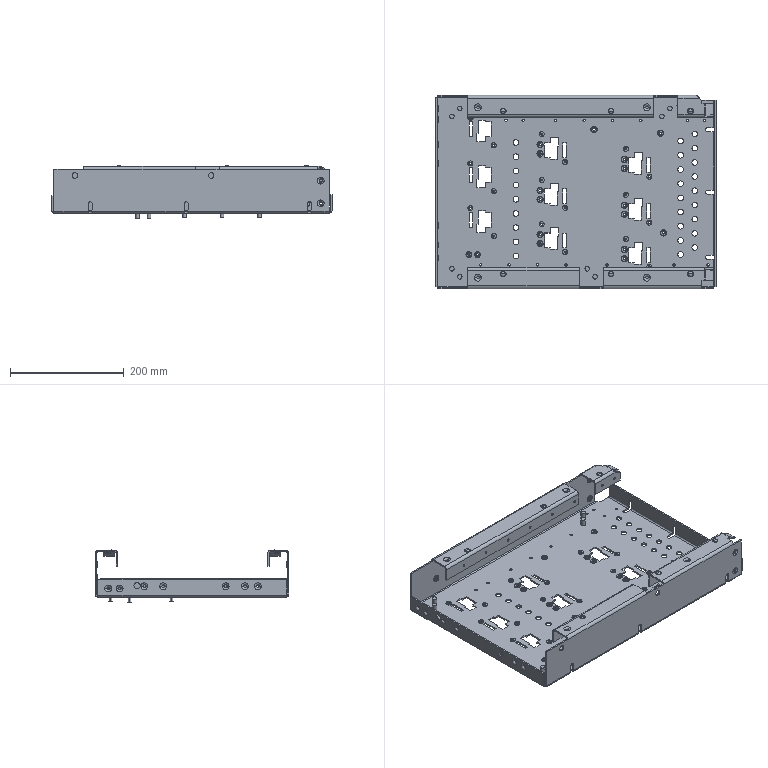Part | STEP file | 64560280 | 1 solid | 1031 faces | box 493.5 x 340.5 x 93 mm | volume 732862 mm3 | cylinder 432 | plane 311 | torus 260 | sphere 24 | spline 4 | commonest cylinder face diameters 10 x104 4.2 x92 5 x46 3.5 x34 8.5 x34 9.2 x30